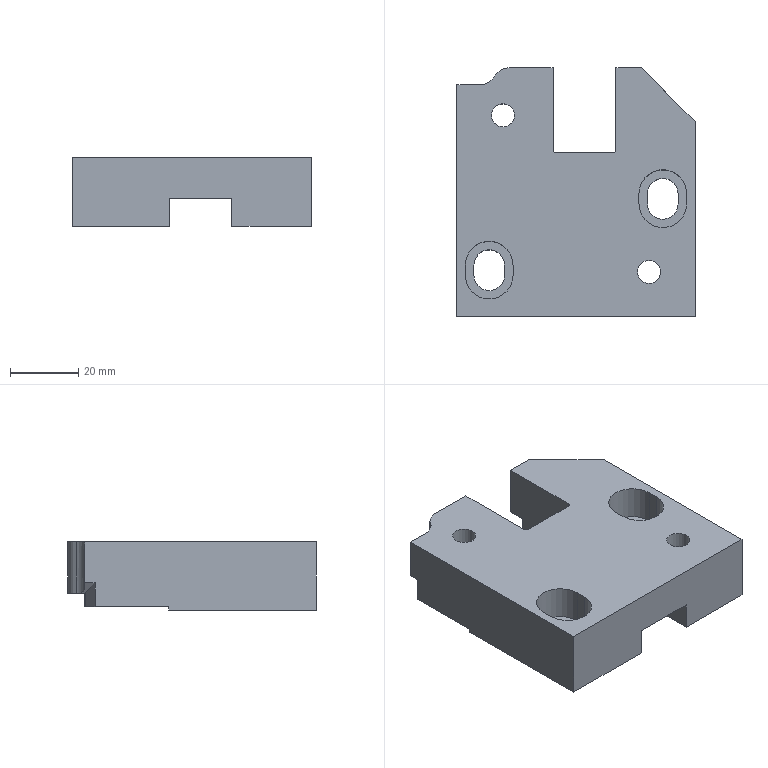Part | NX | features 20 2 | 1 solid | 57 faces | box 70 x 73 x 20 mm | volume 68497 mm3 | plane 39 | cylinder 18 | commonest cylinder face diameters 9 x5 14 x4 10 x3 2 x2 6.8 x2 15 x2